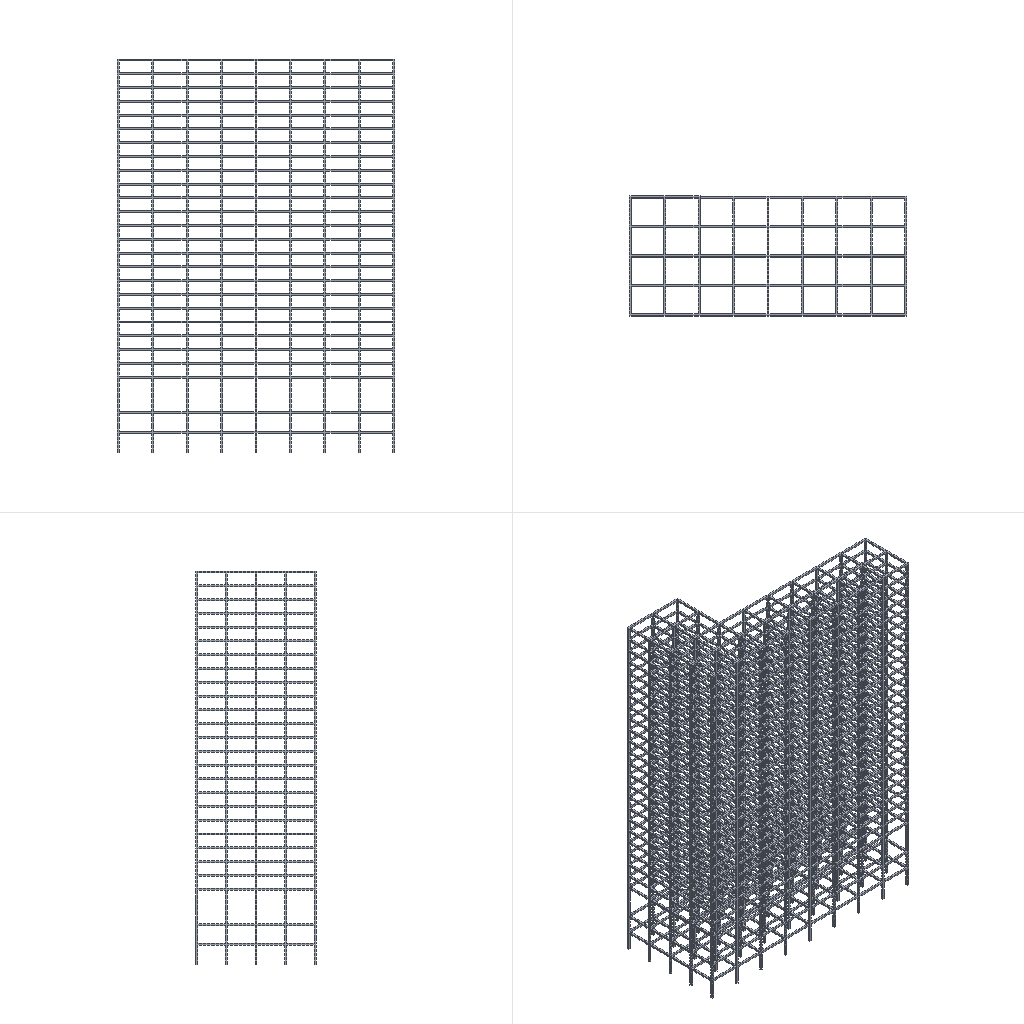Simulation study | abaqus
Set-up summary:
category,name,step,type,value,unit,region
solver,abaqus
solver,version,,,Abaqus/Standard 2020
units,not stated in the deck,,not stated
analysis,deck,,modal,modal
load_step,Step-1,Step-1,modal
load_step,requested,,,1
mesh,nodes,,,53516
mesh,elements,,,14758
element_type,C3D8R,,solid,14758
load,load commands in deck,,count,0
bc,support commands in deck,,count,1
material,MATERIAL-1,,in results
check,setup vs results,,match,"per instance, exact: element labels, types and connectivity; labels of the nodes the elements use; coordinates of those nodes at SINGLE_PRECISION in 1 of 1 instance(s)"
Abaqus input file, long lists of numbers shortened:
*Heading
** Job name: Job-ff Model name: [REDACTED]
** Generated by: Abaqus/CAE 2020
*Preprint, echo=NO, model=NO, history=NO, contact=NO
**
** PARTS
**
*Part, name=Part-1
*Node
      1,        6600.,       18000.,       79600.
      2,        6600.,       17600.,       79600.
** (53514 more lines like these left out)
*Element, type=C3D8R
1,    8,    5, 7348, 7349,    1,    2, 7328, 7341
2, 7349, 7348, 7347, 7350, 7341, 7328, 7329, 7340
** (14756 more lines like these left out)
*Nset, nset=Set-2, generate
     1,  53516,      1
*Elset, elset=Set-2, generate
     1,  14758,      1
** Section: Section-1
*Solid Section, elset=Set-2, material=Material-1
,
*End Part
**
**
** ASSEMBLY
**
*Assembly, name=Assembly
**
*Instance, name=Part-1-1, part=Part-1
*End Instance
**
*Nset, nset=Set-1, instance=Part-1-1
 6187, 6188, 6190, 6191, 6203, 6204, 6206, 6207, 6219, 6220, 6222, 6223, 6235, 6236, 6238, 6239
 6251, 6252, 6254, 6255, 6267, 6268, 6270, 6271, 6283, 6284, 6286, 6287, 6299, 6300, 6302, 6303
** (10 more lines like these left out)
*Elset, elset=Set-1, instance=Part-1-1
  9160,  9170,  9180,  9190,  9200,  9210,  9220,  9230, 10418, 10439, 10460, 10481, 10502, 10523, 10544, 10565
 10642, 10663, 10684, 10705, 10726, 10747, 10768, 10789, 10866, 10887, 10908, 10929, 10950, 10971, 10992, 11013
** (1 more lines like these left out)
*End Assembly
**
** MATERIALS
**
*Material, name=Material-1
*Density
 2.2e-09,
*Elastic
29791., 0.2
*Concrete Damaged Plasticity
30.,    0.1,   1.16, 0.6667,   0.05
*Concrete Compression Hardening
 15.4,      0.
 16.9,  0.0002
 19.6, 0.00048
 20.1, 0.00079
  20., 0.00095
 19.6,  0.0011
 19.1, 0.00127
 18.6, 0.00143
 17.9,  0.0016
 17.2, 0.00177
 16.6, 0.00194
 15.9, 0.00211
 15.3, 0.00228
 14.7, 0.00245
 14.1, 0.00261
 13.5, 0.00278
  13., 0.00294
 12.5,  0.0031
  12., 0.00327
 11.6, 0.00343
 11.2, 0.00359
 10.8, 0.00375
 10.4, 0.00391
 10.1, 0.00406
*Concrete Tension Stiffening
 2.06,      0.
 1.92,   2e-05
 1.72,   4e-05
 1.53,   6e-05
 1.37,   8e-05
 1.24,  0.0001
 1.13, 0.00011
 1.04, 0.00013
 0.97, 0.00015
  0.9, 0.00016
 0.85, 0.00018
*Concrete Compression Damage
     0.,      0.
 0.0841,   9e-05
 0.0933,  0.0001
 0.1091, 0.00013
 0.1418,  0.0002
 0.2407, 0.00048
  0.322, 0.00079
 0.3557, 0.00095
 0.3886,  0.0011
 0.4201, 0.00127
 0.4499, 0.00143
 0.4778,  0.0016
 0.5039, 0.00177
 0.5282, 0.00194
 0.5506, 0.00211
 0.5715, 0.00228
 0.5908, 0.00245
 0.6086, 0.00261
 0.6252, 0.00278
 0.6406, 0.00294
 0.6549,  0.0031
 0.6682, 0.00327
 0.6806, 0.00343
 0.6922, 0.00359
  0.703, 0.00375
 0.7131, 0.00391
 0.7227, 0.00406
   0.74, 0.00438
 0.7554, 0.00469
 0.7691,   0.005
 0.7815, 0.00531
 0.7926, 0.00561
 0.8026, 0.00592
 0.8118, 0.00622
 0.8202, 0.00653
 0.8278, 0.00683
 0.8349, 0.00713
*Concrete Tension Damage
      0.,      0.
 0.1181,   2e-05
 0.2281,   4e-05
 0.3187,   6e-05
 0.3919,   8e-05
 0.4512,  0.0001
 0.5, 0.00011
  0.5407, 0.00013
 0.575, 0.00015
 0.6043, 0.00016
 0.6297, 0.00018
 0.7177, 0.00025
 0.7702, 0.00033
 0.8053,  0.0004
 0.8304, 0.00047
 0.8494, 0.00054
  0.8643, 0.00061
 0.8763, 0.00068
 0.8862, 0.00075
** ----------------------------------------------------------------
**
** STEP: Step-1
**
*Step, name=Step-1, nlgeom=NO, perturbation
*Frequency, eigensolver=Lanczos, sim, acoustic coupling=on, normalization=mass
8, , , , ,
**
** BOUNDARY CONDITIONS
**
** Name: BC-1 Type: 对称/反对称/完全固定
*Boundary
Set-1, PINNED
**
** OUTPUT REQUESTS
**
*Restart, write, frequency=0
**
** FIELD OUTPUT: F-Output-1
**
*Output, field, variable=PRESELECT
*End Step
Results summary:
result,step,,partial,increments=0 time=0.0/1e-36
result,analysis,,,modal
result,last_loadstep,,,1
result,primary field,,,U